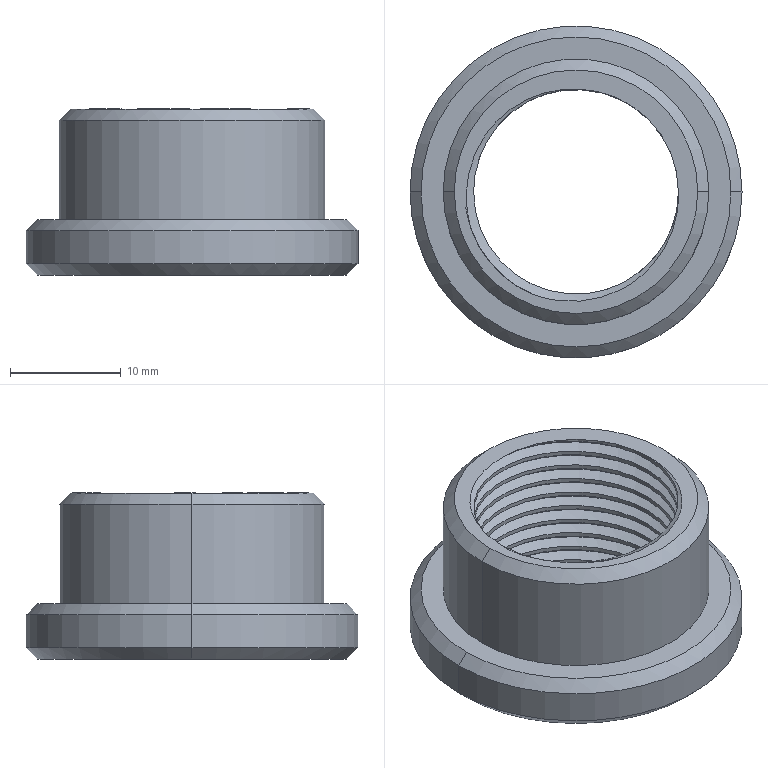Part | SolidWorks | features ICE 2, Chamfer 1, Extrusion 1, SweepThread 1 | 1 solid | 39 faces | box 30 x 30 x 15 mm | volume 3564 mm3 | cylinder 24 | cone 8 | plane 4 | spline 3 | commonest cylinder face diameters 18.5 x20 24 x2 30 x2